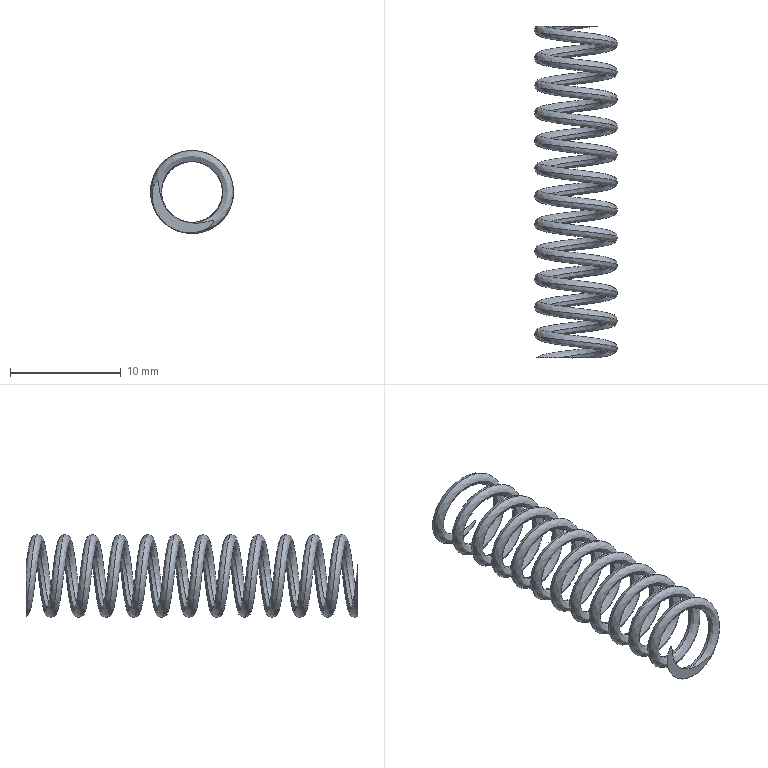Part | SolidWorks | features Helix 1, ICE 1, RefAxis 1, Sweep 1 | 1 solid | 4 faces | box 7.5 x 30 x 7.5 mm | volume 192.185 mm3 | spline 2 | plane 2